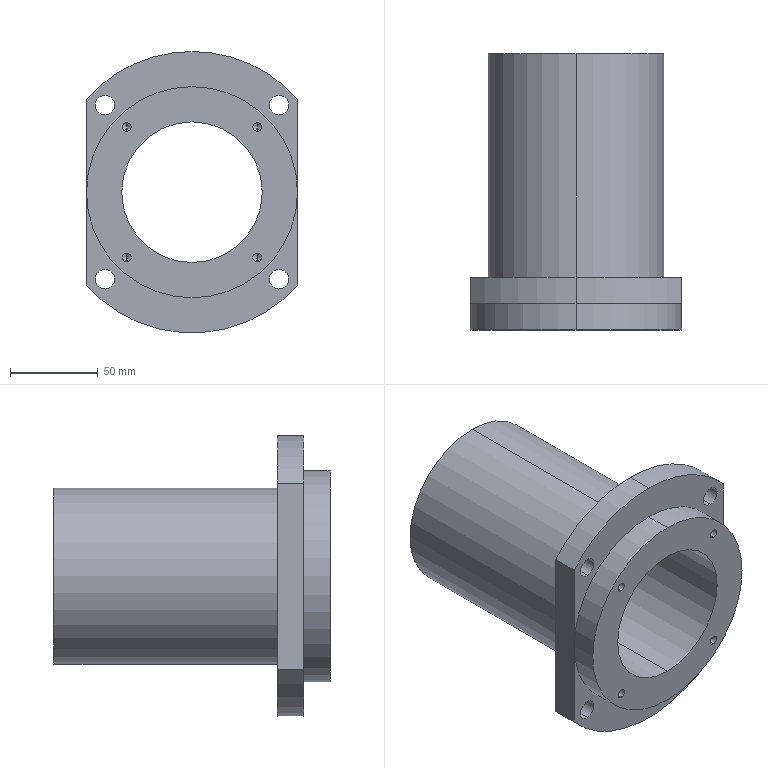Part | STEP file | 0229_210_Holder | 1 solid | 40 faces | box 120 x 157 x 160 mm | volume 628932 mm3 | cylinder 25 | cone 8 | plane 7 | commonest cylinder face diameters 5 x8 11 x8 160 x3 80 x2 100 x2 120 x2